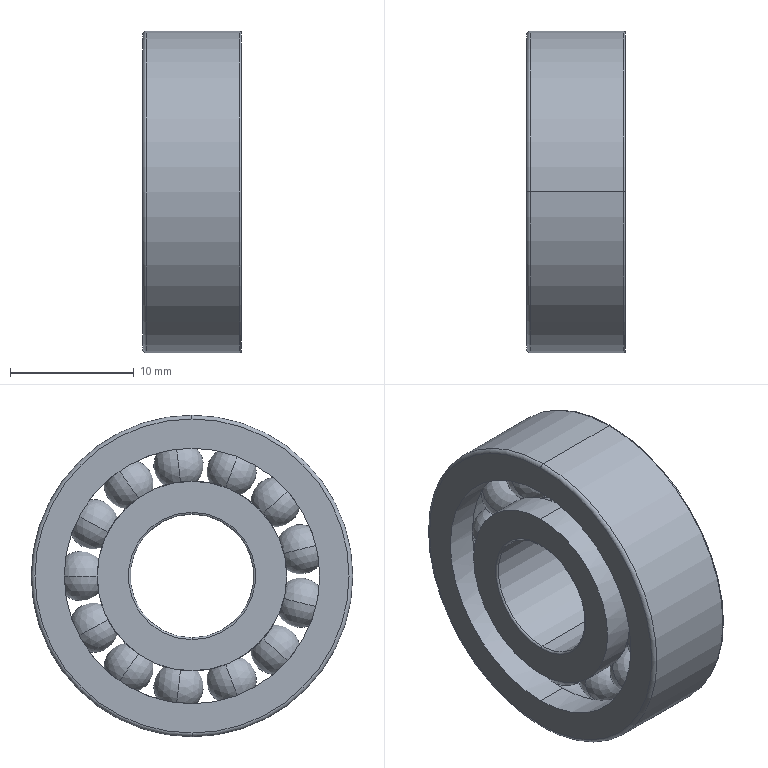Part | NX | 1 solid | 95 faces | box 8 x 26 x 26 mm | volume 2622 mm3 | torus 50 | sphere 26 | cylinder 14 | plane 5 | commonest cylinder face diameters 15.333 x4 10 x2 20.667 x2 21.287 x2 22.287 x2 26 x2